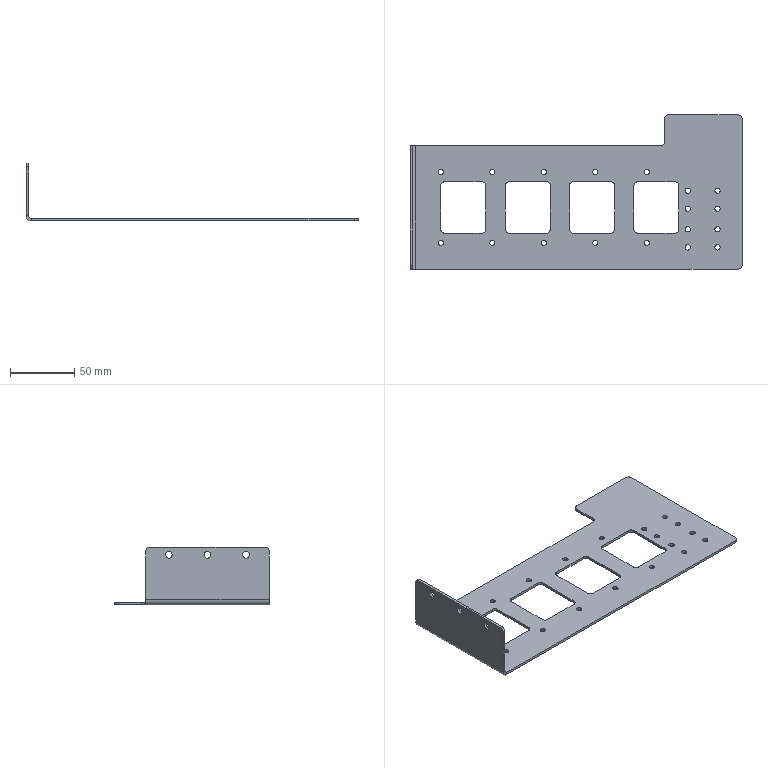Part | STEP file | SynoNew-0304-064 | 1 solid | 73 faces | box 258 x 120 x 45 mm | volume 48671 mm3 | cylinder 45 | plane 28 | commonest cylinder face diameters 6 x22 4 x11 4.2 x8 5.2 x3 8 x1